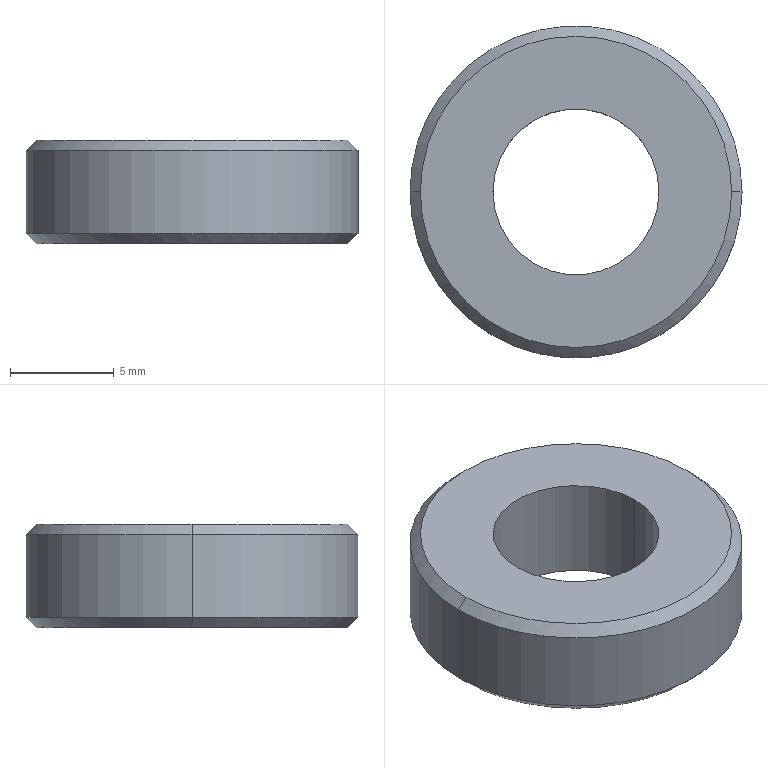Part | SolidWorks | features Chamfer 1, Extrusion 1 | 1 solid | 10 faces | box 16 x 16 x 5 mm | volume 741.678 mm3 | cone 4 | cylinder 4 | plane 2 | commonest cylinder face diameters 8 x2 16 x2
STEP:
#1=CARTESIAN_POINT('',(7.5,0.,2.5));
#2=VERTEX_POINT('',#1);
#3=CARTESIAN_POINT('',(-7.5,0.,2.5));
#4=VERTEX_POINT('',#3);
#5=CARTESIAN_POINT('',(0.,0.,2.5));
#6=DIRECTION('',(0.,0.,1.));
#7=DIRECTION('',(1.,0.,0.));
#8=AXIS2_PLACEMENT_3D('',#5,#6,#7);
#9=CIRCLE('',#8,7.5);
#10=EDGE_CURVE('',#2,#4,#9,.T.);
#11=ORIENTED_EDGE('',*,*,#10,.F.);
#12=CARTESIAN_POINT('',(8.,0.,2.));
#13=VERTEX_POINT('',#12);
#14=CARTESIAN_POINT('',(7.5,0.,2.5));
#15=DIRECTION('',(0.7071,0.,-0.7071));
#16=VECTOR('',#15,1000.);
#17=LINE('',#14,#16);
#18=EDGE_CURVE('',#2,#13,#17,.T.);
#19=ORIENTED_EDGE('',*,*,#18,.T.);
#20=CARTESIAN_POINT('',(-8.,0.,2.));
#21=VERTEX_POINT('',#20);
#22=CARTESIAN_POINT('',(0.,0.,2.));
#23=DIRECTION('',(0.,0.,-1.));
#24=DIRECTION('',(1.,0.,0.));
#25=AXIS2_PLACEMENT_3D('',#22,#23,#24);
#26=CIRCLE('',#25,8.);
#27=EDGE_CURVE('',#21,#13,#26,.T.);
#28=ORIENTED_EDGE('',*,*,#27,.F.);
#29=CARTESIAN_POINT('',(-7.5,0.,2.5));
#30=DIRECTION('',(-0.7071,0.,-0.7071));
#31=VECTOR('',#30,1000.);
#32=LINE('',#29,#31);
#33=EDGE_CURVE('',#4,#21,#32,.T.);
#34=ORIENTED_EDGE('',*,*,#33,.F.);
#35=EDGE_LOOP('',(#11,#19,#28,#34));
#36=FACE_OUTER_BOUND('',#35,.T.);
#37=CARTESIAN_POINT('',(0.,0.,2.5));
#38=DIRECTION('',(0.,0.,-1.));
#39=DIRECTION('',(-1.,0.,0.));
#40=AXIS2_PLACEMENT_3D('',#37,#38,#39);
#41=CONICAL_SURFACE('',#40,7.5,0.7854);
#42=ADVANCED_FACE('',(#36),#41,.T.);
#43=CARTESIAN_POINT('',(-7.5,0.,-2.5));
#44=VERTEX_POINT('',#43);
#45=CARTESIAN_POINT('',(7.5,0.,-2.5));
#46=VERTEX_POINT('',#45);
#47=CARTESIAN_POINT('',(0.,0.,-2.5));
#48=DIRECTION('',(0.,0.,-1.));
#49=DIRECTION('',(1.,0.,0.));
#50=AXIS2_PLACEMENT_3D('',#47,#48,#49);
#51=CIRCLE('',#50,7.5);
#52=EDGE_CURVE('',#44,#46,#51,.T.);
#53=ORIENTED_EDGE('',*,*,#52,.F.);
#54=CARTESIAN_POINT('',(-8.,0.,-2.));
#55=VERTEX_POINT('',#54);
#56=CARTESIAN_POINT('',(-8.,0.,-2.));
#57=DIRECTION('',(-0.7071,0.,0.7071));
#58=VECTOR('',#57,1000.);
#59=LINE('',#56,#58);
#60=EDGE_CURVE('',#44,#55,#59,.T.);
#61=ORIENTED_EDGE('',*,*,#60,.T.);
#62=CARTESIAN_POINT('',(8.,0.,-2.));
#63=VERTEX_POINT('',#62);
#64=CARTESIAN_POINT('',(0.,0.,-2.));
#65=DIRECTION('',(0.,0.,1.));
#66=DIRECTION('',(1.,0.,0.));
#67=AXIS2_PLACEMENT_3D('',#64,#65,#66);
#68=CIRCLE('',#67,8.);
#69=EDGE_CURVE('',#63,#55,#68,.T.);
#70=ORIENTED_EDGE('',*,*,#69,.F.);
#71=CARTESIAN_POINT('',(8.,0.,-2.));
#72=DIRECTION('',(0.7071,0.,0.7071));
#73=VECTOR('',#72,1000.);
#74=LINE('',#71,#73);
#75=EDGE_CURVE('',#46,#63,#74,.T.);
#76=ORIENTED_EDGE('',*,*,#75,.F.);
#77=EDGE_LOOP('',(#53,#61,#70,#76));
#78=FACE_OUTER_BOUND('',#77,.T.);
#79=CARTESIAN_POINT('',(0.,0.,-2.));
#80=DIRECTION('',(0.,0.,1.));
#81=DIRECTION('',(1.,0.,0.));
#82=AXIS2_PLACEMENT_3D('',#79,#80,#81);
#83=CONICAL_SURFACE('',#82,8.,0.7854);
#84=ADVANCED_FACE('',(#78),#83,.T.);
#85=CARTESIAN_POINT('',(-4.,0.,2.5));
#86=VERTEX_POINT('',#85);
#87=CARTESIAN_POINT('',(4.,0.,2.5));
#88=VERTEX_POINT('',#87);
#89=CARTESIAN_POINT('',(0.,0.,2.5));
#90=DIRECTION('',(0.,0.,1.));
#91=DIRECTION('',(1.,0.,0.));
#92=AXIS2_PLACEMENT_3D('',#89,#90,#91);
#93=CIRCLE('',#92,4.);
#94=EDGE_CURVE('',#86,#88,#93,.T.);
#95=ORIENTED_EDGE('',*,*,#94,.T.);
#96=CARTESIAN_POINT('',(4.,0.,-2.5));
#97=VERTEX_POINT('',#96);
#98=CARTESIAN_POINT('',(4.,0.,2.5));
#99=DIRECTION('',(0.,0.,-1.));
#100=VECTOR('',#99,1000.);
#101=LINE('',#98,#100);
#102=EDGE_CURVE('',#88,#97,#101,.T.);
#103=ORIENTED_EDGE('',*,*,#102,.T.);
#104=CARTESIAN_POINT('',(-4.,0.,-2.5));
#105=VERTEX_POINT('',#104);
#106=CARTESIAN_POINT('',(0.,0.,-2.5));
#107=DIRECTION('',(0.,0.,1.));
#108=DIRECTION('',(1.,0.,0.));
#109=AXIS2_PLACEMENT_3D('',#106,#107,#108);
#110=CIRCLE('',#109,4.);
#111=EDGE_CURVE('',#105,#97,#110,.T.);
#112=ORIENTED_EDGE('',*,*,#111,.F.);
#113=CARTESIAN_POINT('',(-4.,0.,2.5));
#114=DIRECTION('',(0.,0.,-1.));
#115=VECTOR('',#114,1000.);
#116=LINE('',#113,#115);
#117=EDGE_CURVE('',#86,#105,#116,.T.);
#118=ORIENTED_EDGE('',*,*,#117,.F.);
#119=EDGE_LOOP('',(#95,#103,#112,#118));
#120=FACE_OUTER_BOUND('',#119,.T.);
#121=CARTESIAN_POINT('',(0.,0.,2.5));
#122=DIRECTION('',(0.,0.,-1.));
#123=DIRECTION('',(-1.,0.,0.));
#124=AXIS2_PLACEMENT_3D('',#121,#122,#123);
#125=CYLINDRICAL_SURFACE('',#124,4.);
#126=ADVANCED_FACE('',(#120),#125,.F.);
#127=ORIENTED_EDGE('',*,*,#27,.T.);
#128=CARTESIAN_POINT('',(8.,0.,2.5));
#129=DIRECTION('',(0.,0.,-1.));
#130=VECTOR('',#129,1000.);
#131=LINE('',#128,#130);
#132=EDGE_CURVE('',#13,#63,#131,.T.);
#133=ORIENTED_EDGE('',*,*,#132,.T.);
#134=ORIENTED_EDGE('',*,*,#69,.T.);
#135=CARTESIAN_POINT('',(-8.,0.,2.5));
#136=DIRECTION('',(0.,0.,-1.));
#137=VECTOR('',#136,1000.);
#138=LINE('',#135,#137);
#139=EDGE_CURVE('',#21,#55,#138,.T.);
#140=ORIENTED_EDGE('',*,*,#139,.F.);
#141=EDGE_LOOP('',(#127,#133,#134,#140));
#142=FACE_OUTER_BOUND('',#141,.T.);
#143=CARTESIAN_POINT('',(0.,0.,2.5));
#144=DIRECTION('',(0.,0.,-1.));
#145=DIRECTION('',(-1.,0.,0.));
#146=AXIS2_PLACEMENT_3D('',#143,#144,#145);
#147=CYLINDRICAL_SURFACE('',#146,8.);
#148=ADVANCED_FACE('',(#142),#147,.T.);
#149=CARTESIAN_POINT('',(0.,0.,2.5));
#150=DIRECTION('',(0.,0.,1.));
#151=DIRECTION('',(1.,0.,0.));
#152=AXIS2_PLACEMENT_3D('',#149,#150,#151);
#153=CIRCLE('',#152,7.5);
#154=EDGE_CURVE('',#4,#2,#153,.T.);
#155=ORIENTED_EDGE('',*,*,#154,.T.);
#156=ORIENTED_EDGE('',*,*,#10,.T.);
#157=EDGE_LOOP('',(#155,#156));
#158=FACE_OUTER_BOUND('',#157,.T.);
#159=ORIENTED_EDGE('',*,*,#94,.F.);
#160=CARTESIAN_POINT('',(0.,0.,2.5));
#161=DIRECTION('',(0.,0.,1.));
#162=DIRECTION('',(1.,0.,0.));
#163=AXIS2_PLACEMENT_3D('',#160,#161,#162);
#164=CIRCLE('',#163,4.);
#165=EDGE_CURVE('',#88,#86,#164,.T.);
#166=ORIENTED_EDGE('',*,*,#165,.F.);
#167=EDGE_LOOP('',(#159,#166));
#168=FACE_BOUND('',#167,.T.);
#169=CARTESIAN_POINT('',(0.,0.,2.5));
#170=DIRECTION('',(0.,0.,1.));
#171=DIRECTION('',(1.,0.,0.));
#172=AXIS2_PLACEMENT_3D('',#169,#170,#171);
#173=PLANE('',#172);
#174=ADVANCED_FACE('',(#158,#168),#173,.T.);
#175=CARTESIAN_POINT('',(0.,0.,-2.5));
#176=DIRECTION('',(0.,0.,-1.));
#177=DIRECTION('',(1.,0.,0.));
#178=AXIS2_PLACEMENT_3D('',#175,#176,#177);
#179=CIRCLE('',#178,7.5);
#180=EDGE_CURVE('',#46,#44,#179,.T.);
#181=ORIENTED_EDGE('',*,*,#180,.T.);
#182=ORIENTED_EDGE('',*,*,#52,.T.);
#183=EDGE_LOOP('',(#181,#182));
#184=FACE_OUTER_BOUND('',#183,.T.);
#185=ORIENTED_EDGE('',*,*,#111,.T.);
#186=CARTESIAN_POINT('',(0.,0.,-2.5));
#187=DIRECTION('',(0.,0.,1.));
#188=DIRECTION('',(1.,0.,0.));
#189=AXIS2_PLACEMENT_3D('',#186,#187,#188);
#190=CIRCLE('',#189,4.);
#191=EDGE_CURVE('',#97,#105,#190,.T.);
#192=ORIENTED_EDGE('',*,*,#191,.T.);
#193=EDGE_LOOP('',(#185,#192));
#194=FACE_BOUND('',#193,.T.);
#195=CARTESIAN_POINT('',(0.,0.,-2.5));
#196=DIRECTION('',(0.,0.,1.));
#197=DIRECTION('',(1.,0.,0.));
#198=AXIS2_PLACEMENT_3D('',#195,#196,#197);
#199=PLANE('',#198);
#200=ADVANCED_FACE('',(#184,#194),#199,.F.);
#201=ORIENTED_EDGE('',*,*,#132,.F.);
#202=CARTESIAN_POINT('',(0.,0.,2.));
#203=DIRECTION('',(0.,0.,-1.));
#204=DIRECTION('',(1.,0.,0.));
#205=AXIS2_PLACEMENT_3D('',#202,#203,#204);
#206=CIRCLE('',#205,8.);
#207=EDGE_CURVE('',#13,#21,#206,.T.);
#208=ORIENTED_EDGE('',*,*,#207,.T.);
#209=ORIENTED_EDGE('',*,*,#139,.T.);
#210=CARTESIAN_POINT('',(0.,0.,-2.));
#211=DIRECTION('',(0.,0.,1.));
#212=DIRECTION('',(1.,0.,0.));
#213=AXIS2_PLACEMENT_3D('',#210,#211,#212);
#214=CIRCLE('',#213,8.);
#215=EDGE_CURVE('',#55,#63,#214,.T.);
#216=ORIENTED_EDGE('',*,*,#215,.T.);
#217=EDGE_LOOP('',(#201,#208,#209,#216));
#218=FACE_OUTER_BOUND('',#217,.T.);
#219=CARTESIAN_POINT('',(0.,0.,2.5));
#220=DIRECTION('',(0.,0.,-1.));
#221=DIRECTION('',(-1.,0.,0.));
#222=AXIS2_PLACEMENT_3D('',#219,#220,#221);
#223=CYLINDRICAL_SURFACE('',#222,8.);
#224=ADVANCED_FACE('',(#218),#223,.T.);
#225=ORIENTED_EDGE('',*,*,#102,.F.);
#226=ORIENTED_EDGE('',*,*,#165,.T.);
#227=ORIENTED_EDGE('',*,*,#117,.T.);
#228=ORIENTED_EDGE('',*,*,#191,.F.);
#229=EDGE_LOOP('',(#225,#226,#227,#228));
#230=FACE_OUTER_BOUND('',#229,.T.);
#231=CARTESIAN_POINT('',(0.,0.,2.5));
#232=DIRECTION('',(0.,0.,-1.));
#233=DIRECTION('',(-1.,0.,0.));
#234=AXIS2_PLACEMENT_3D('',#231,#232,#233);
#235=CYLINDRICAL_SURFACE('',#234,4.);
#236=ADVANCED_FACE('',(#230),#235,.F.);
#237=ORIENTED_EDGE('',*,*,#60,.F.);
#238=ORIENTED_EDGE('',*,*,#180,.F.);
#239=ORIENTED_EDGE('',*,*,#75,.T.);
#240=ORIENTED_EDGE('',*,*,#215,.F.);
#241=EDGE_LOOP('',(#237,#238,#239,#240));
#242=FACE_OUTER_BOUND('',#241,.T.);
#243=CARTESIAN_POINT('',(0.,0.,-2.));
#244=DIRECTION('',(0.,0.,1.));
#245=DIRECTION('',(1.,0.,0.));
#246=AXIS2_PLACEMENT_3D('',#243,#244,#245);
#247=CONICAL_SURFACE('',#246,8.,0.7854);
#248=ADVANCED_FACE('',(#242),#247,.T.);
#249=ORIENTED_EDGE('',*,*,#18,.F.);
#250=ORIENTED_EDGE('',*,*,#154,.F.);
#251=ORIENTED_EDGE('',*,*,#33,.T.);
#252=ORIENTED_EDGE('',*,*,#207,.F.);
#253=EDGE_LOOP('',(#249,#250,#251,#252));
#254=FACE_OUTER_BOUND('',#253,.T.);
#255=CARTESIAN_POINT('',(0.,0.,2.5));
#256=DIRECTION('',(0.,0.,-1.));
#257=DIRECTION('',(-1.,0.,0.));
#258=AXIS2_PLACEMENT_3D('',#255,#256,#257);
#259=CONICAL_SURFACE('',#258,7.5,0.7854);
#260=ADVANCED_FACE('',(#254),#259,.T.);
#261=CLOSED_SHELL('',(#42,#84,#126,#148,#174,#200,#224,#236,#248,#260));
#262=MANIFOLD_SOLID_BREP('',#261);
#263=CARTESIAN_POINT('',(0.,0.,0.));
#264=DIRECTION('',(0.,0.,1.));
#265=DIRECTION('',(1.,0.,0.));
#266=AXIS2_PLACEMENT_3D('',#263,#264,#265);
#267=(LENGTH_UNIT()NAMED_UNIT(*)SI_UNIT(.MILLI.,.METRE.));
#268=UNCERTAINTY_MEASURE_WITH_UNIT(LENGTH_MEASURE(0.00001),#267,'','');
#269=(NAMED_UNIT(*)PLANE_ANGLE_UNIT()SI_UNIT($,.RADIAN.));
#270=(NAMED_UNIT(*)SI_UNIT($,.STERADIAN.)SOLID_ANGLE_UNIT());
#271=(GEOMETRIC_REPRESENTATION_CONTEXT(3)GLOBAL_UNCERTAINTY_ASSIGNED_CONTEXT((#268))GLOBAL_UNIT_ASSIGNED_CONTEXT((#267,#269,#270))REPRESENTATION_CONTEXT('',''));
#272=ADVANCED_BREP_SHAPE_REPRESENTATION('',(#262,#266),#271);